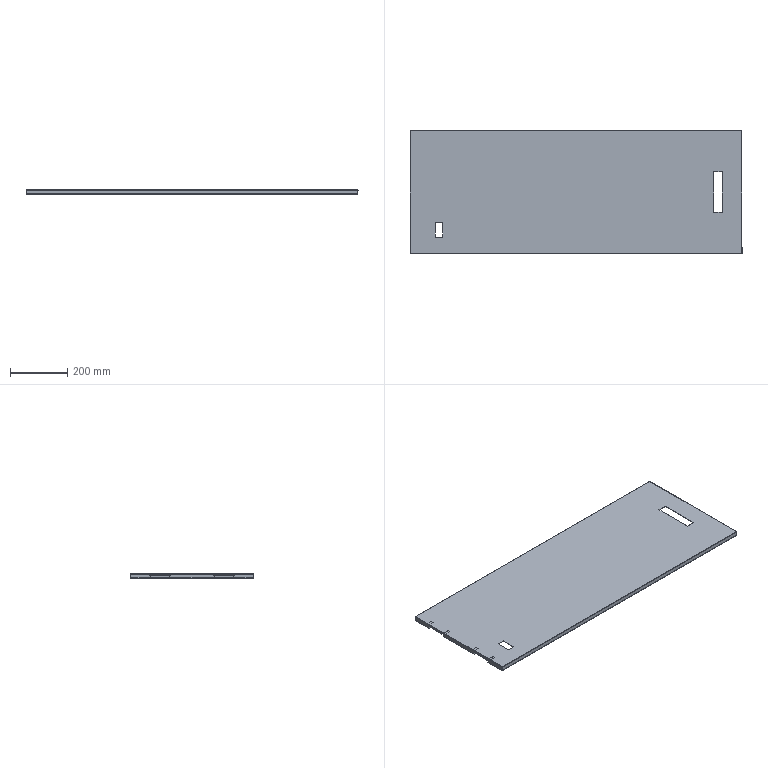Part | NX | features BREP 3 | 3 solids | 182 faces | box 1160 x 432 x 16.5 mm | volume 853876 mm3 | plane 118 | cylinder 48 | spline 16 | commonest cylinder face diameters 0.02 x18 3.02 x18 3.2 x12